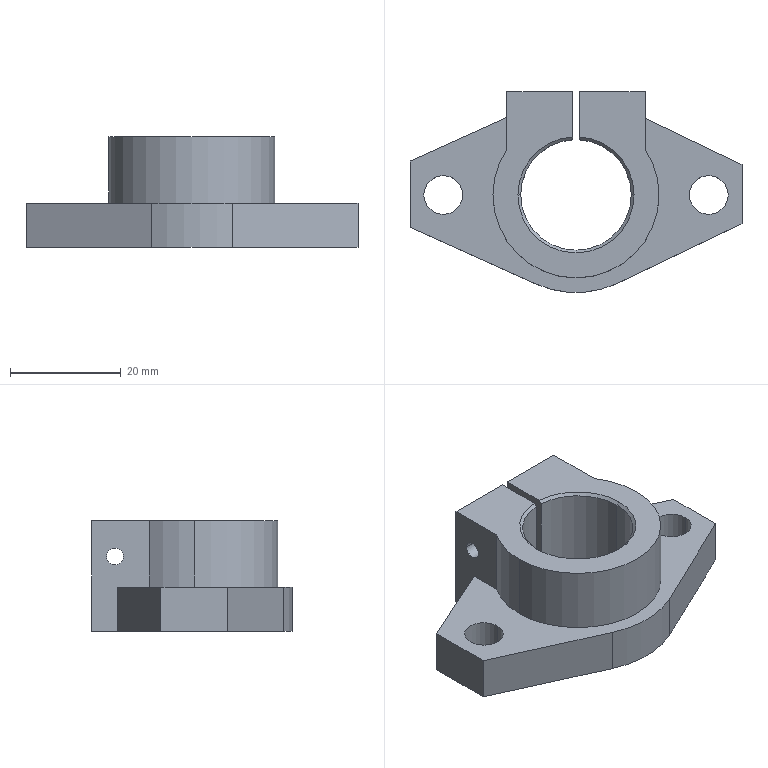Part | STEP file | SHF20 | 1 solid | 36 faces | box 60 x 36.276 x 20 mm | volume 15283 mm3 | cylinder 15 | plane 15 | cone 6 | commonest cylinder face diameters 3 x4 7 x4 20 x3 30 x3 35.27 x1